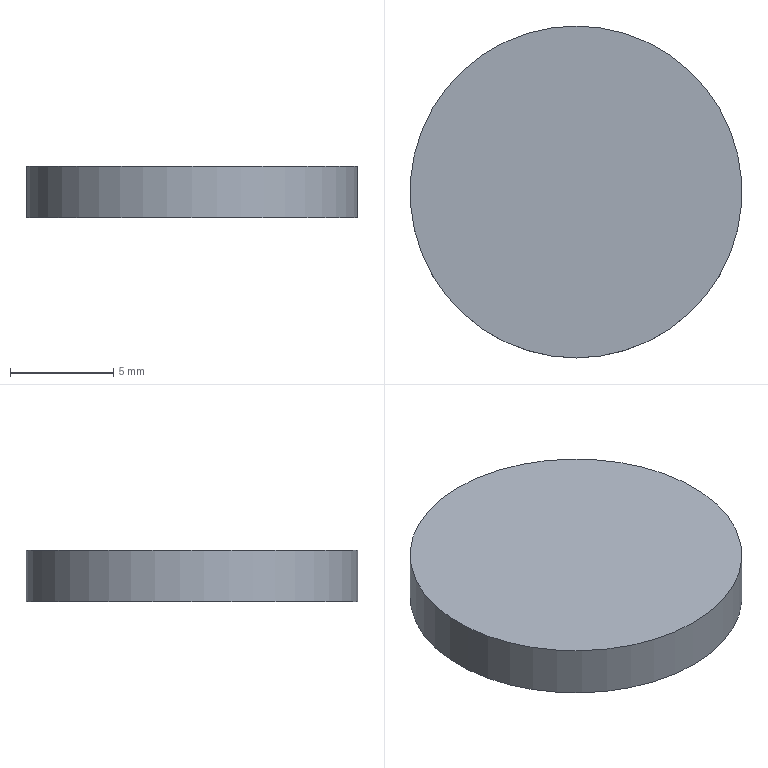Part | STEP file | lll_id1314_x_t | 1 solid | 3 faces | box 16.07 x 16.07 x 2.5 mm | volume 507.063 mm3 | plane 2 | cylinder 1 | commonest cylinder face diameters 16.07 x1
STEP:
#1=CARTESIAN_POINT('',(3364.5,67.465,0.00001741));
#2=VERTEX_POINT('',#1);
#3=CARTESIAN_POINT('',(3364.5,75.5,0.00001741));
#4=DIRECTION('',(0.000000008,0.,-1.));
#5=DIRECTION('',(0.,-1.,0.));
#6=AXIS2_PLACEMENT_3D('',#3,#4,#5);
#7=CIRCLE('',#6,8.035);
#8=EDGE_CURVE('',#2,#2,#7,.T.);
#9=ORIENTED_EDGE('',*,*,#8,.T.);
#10=EDGE_LOOP('',(#9));
#11=FACE_OUTER_BOUND('',#10,.T.);
#12=CARTESIAN_POINT('',(3364.5,75.5,0.00001741));
#13=DIRECTION('',(0.000000008,0.,-1.));
#14=DIRECTION('',(0.,-1.,0.));
#15=AXIS2_PLACEMENT_3D('',#12,#13,#14);
#16=PLANE('',#15);
#17=ADVANCED_FACE('',(#11),#16,.T.);
#18=CARTESIAN_POINT('',(3364.5,67.465,2.5));
#19=VERTEX_POINT('',#18);
#20=CARTESIAN_POINT('',(3364.5,75.5,2.5));
#21=DIRECTION('',(0.000000008,0.,-1.));
#22=DIRECTION('',(0.,-1.,0.));
#23=AXIS2_PLACEMENT_3D('',#20,#21,#22);
#24=CIRCLE('',#23,8.035);
#25=EDGE_CURVE('',#19,#19,#24,.T.);
#26=ORIENTED_EDGE('',*,*,#25,.F.);
#27=EDGE_LOOP('',(#26));
#28=FACE_OUTER_BOUND('',#27,.T.);
#29=CARTESIAN_POINT('',(3364.5,75.5,2.5));
#30=DIRECTION('',(-0.000000008,0.,1.));
#31=DIRECTION('',(0.,1.,0.));
#32=AXIS2_PLACEMENT_3D('',#29,#30,#31);
#33=PLANE('',#32);
#34=ADVANCED_FACE('',(#28),#33,.T.);
#35=ORIENTED_EDGE('',*,*,#8,.F.);
#36=EDGE_LOOP('',(#35));
#37=FACE_BOUND('',#36,.T.);
#38=ORIENTED_EDGE('',*,*,#25,.T.);
#39=EDGE_LOOP('',(#38));
#40=FACE_BOUND('',#39,.T.);
#41=CARTESIAN_POINT('',(3364.5,75.5,2.5));
#42=DIRECTION('',(0.000000008,0.,-1.));
#43=DIRECTION('',(0.,-1.,0.));
#44=AXIS2_PLACEMENT_3D('',#41,#42,#43);
#45=CYLINDRICAL_SURFACE('',#44,8.035);
#46=ADVANCED_FACE('',(#37,#40),#45,.T.);
#47=CLOSED_SHELL('',(#17,#34,#46));
#48=MANIFOLD_SOLID_BREP('',#47);
#49=(LENGTH_UNIT()NAMED_UNIT(*)SI_UNIT(.MILLI.,.METRE.));
#50=UNCERTAINTY_MEASURE_WITH_UNIT(LENGTH_MEASURE(0.00002),#49,'','');
#51=(NAMED_UNIT(*)PLANE_ANGLE_UNIT()SI_UNIT($,.RADIAN.));
#52=PLANE_ANGLE_MEASURE_WITH_UNIT(PLANE_ANGLE_MEASURE(0.01745),#51);
#53=DIMENSIONAL_EXPONENTS(0.,0.,0.,0.,0.,0.,0.);
#54=(CONVERSION_BASED_UNIT('DEGREE',#52)NAMED_UNIT(#53)PLANE_ANGLE_UNIT());
#55=(NAMED_UNIT(*)SI_UNIT($,.STERADIAN.)SOLID_ANGLE_UNIT());
#56=(GEOMETRIC_REPRESENTATION_CONTEXT(3)GLOBAL_UNCERTAINTY_ASSIGNED_CONTEXT((#50))GLOBAL_UNIT_ASSIGNED_CONTEXT((#49,#54,#55))REPRESENTATION_CONTEXT('',''));
#57=ADVANCED_BREP_SHAPE_REPRESENTATION('',(#48),#56);